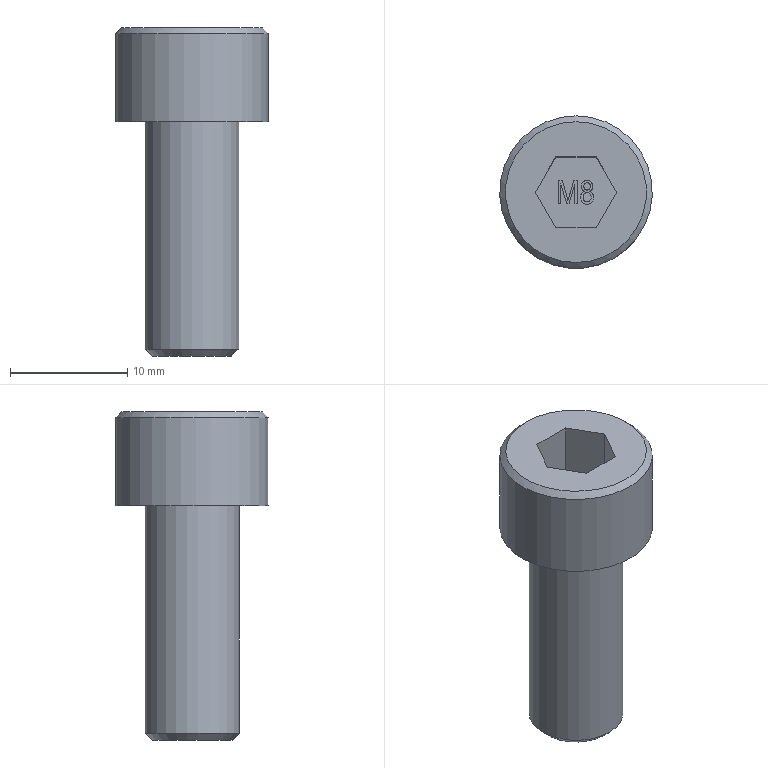Part | STEP file | EM10802000 | 1 solid | 38 faces | box 13 x 13 x 28 mm | volume 1902 mm3 | plane 25 | other 9 | cylinder 2 | cone 2 | commonest cylinder face diameters 8 x1 13 x1